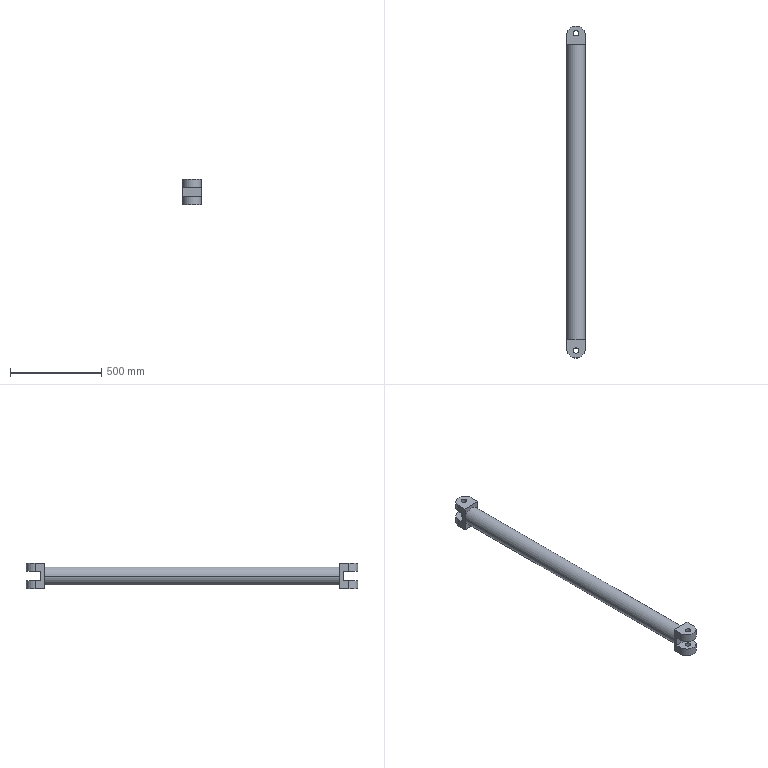Part | STEP file | AX-R-AV | 3 solids | 32 faces | box 100 x 1818 x 140 mm | volume 14387366 mm3 | plane 18 | cylinder 14 | commonest cylinder face diameters 30 x8 100 x6